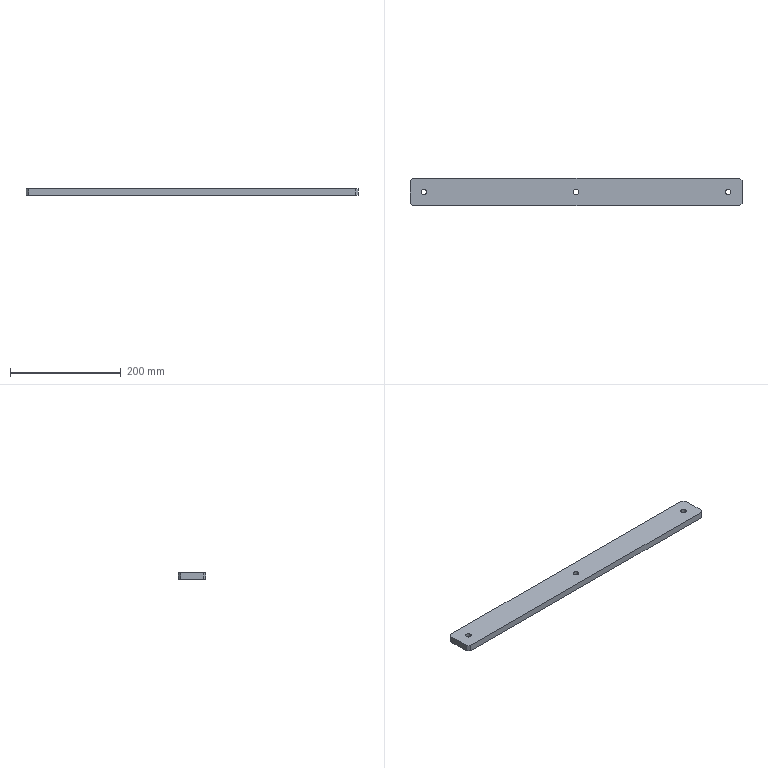Part | STEP file | [16] | 1 solid | 16 faces | box 600 x 50 x 12 mm | volume 356573 mm3 | plane 10 | cylinder 6 | commonest cylinder face diameters 10 x6
STEP:
#1=CARTESIAN_POINT('',(-530.,25.,0.));
#2=VERTEX_POINT('',#1);
#3=CARTESIAN_POINT('',(-520.,25.,0.));
#4=VERTEX_POINT('',#3);
#5=CARTESIAN_POINT('',(-525.,25.,0.));
#6=DIRECTION('',(0.,0.,1.));
#7=DIRECTION('',(1.,0.,0.));
#8=AXIS2_PLACEMENT_3D('',#5,#6,#7);
#9=CIRCLE('',#8,5.);
#10=EDGE_CURVE('',#2,#4,#9,.T.);
#11=ORIENTED_EDGE('',*,*,#10,.F.);
#12=CARTESIAN_POINT('',(-530.,25.,12.));
#13=VERTEX_POINT('',#12);
#14=CARTESIAN_POINT('',(-530.,25.,0.));
#15=DIRECTION('',(0.,0.,1.));
#16=VECTOR('',#15,1000.);
#17=LINE('',#14,#16);
#18=EDGE_CURVE('',#2,#13,#17,.T.);
#19=ORIENTED_EDGE('',*,*,#18,.T.);
#20=CARTESIAN_POINT('',(-520.,25.,12.));
#21=VERTEX_POINT('',#20);
#22=CARTESIAN_POINT('',(-525.,25.,12.));
#23=DIRECTION('',(0.,0.,-1.));
#24=DIRECTION('',(-1.,0.,0.));
#25=AXIS2_PLACEMENT_3D('',#22,#23,#24);
#26=CIRCLE('',#25,5.);
#27=EDGE_CURVE('',#21,#13,#26,.T.);
#28=ORIENTED_EDGE('',*,*,#27,.F.);
#29=CARTESIAN_POINT('',(-520.,25.,0.));
#30=DIRECTION('',(0.,0.,1.));
#31=VECTOR('',#30,1000.);
#32=LINE('',#29,#31);
#33=EDGE_CURVE('',#4,#21,#32,.T.);
#34=ORIENTED_EDGE('',*,*,#33,.F.);
#35=EDGE_LOOP('',(#11,#19,#28,#34));
#36=FACE_OUTER_BOUND('',#35,.T.);
#37=CARTESIAN_POINT('',(-525.,25.,0.));
#38=DIRECTION('',(0.,0.,1.));
#39=DIRECTION('',(1.,0.,0.));
#40=AXIS2_PLACEMENT_3D('',#37,#38,#39);
#41=CYLINDRICAL_SURFACE('',#40,5.);
#42=ADVANCED_FACE('',(#36),#41,.F.);
#43=CARTESIAN_POINT('',(-255.,25.,0.));
#44=VERTEX_POINT('',#43);
#45=CARTESIAN_POINT('',(-245.,25.,0.));
#46=VERTEX_POINT('',#45);
#47=CARTESIAN_POINT('',(-250.,25.,0.));
#48=DIRECTION('',(0.,0.,1.));
#49=DIRECTION('',(1.,0.,0.));
#50=AXIS2_PLACEMENT_3D('',#47,#48,#49);
#51=CIRCLE('',#50,5.);
#52=EDGE_CURVE('',#44,#46,#51,.T.);
#53=ORIENTED_EDGE('',*,*,#52,.F.);
#54=CARTESIAN_POINT('',(-255.,25.,12.));
#55=VERTEX_POINT('',#54);
#56=CARTESIAN_POINT('',(-255.,25.,0.));
#57=DIRECTION('',(0.,0.,1.));
#58=VECTOR('',#57,1000.);
#59=LINE('',#56,#58);
#60=EDGE_CURVE('',#44,#55,#59,.T.);
#61=ORIENTED_EDGE('',*,*,#60,.T.);
#62=CARTESIAN_POINT('',(-245.,25.,12.));
#63=VERTEX_POINT('',#62);
#64=CARTESIAN_POINT('',(-250.,25.,12.));
#65=DIRECTION('',(0.,0.,-1.));
#66=DIRECTION('',(-1.,0.,0.));
#67=AXIS2_PLACEMENT_3D('',#64,#65,#66);
#68=CIRCLE('',#67,5.);
#69=EDGE_CURVE('',#63,#55,#68,.T.);
#70=ORIENTED_EDGE('',*,*,#69,.F.);
#71=CARTESIAN_POINT('',(-245.,25.,0.));
#72=DIRECTION('',(0.,0.,1.));
#73=VECTOR('',#72,1000.);
#74=LINE('',#71,#73);
#75=EDGE_CURVE('',#46,#63,#74,.T.);
#76=ORIENTED_EDGE('',*,*,#75,.F.);
#77=EDGE_LOOP('',(#53,#61,#70,#76));
#78=FACE_OUTER_BOUND('',#77,.T.);
#79=CARTESIAN_POINT('',(-250.,25.,0.));
#80=DIRECTION('',(0.,0.,1.));
#81=DIRECTION('',(1.,0.,0.));
#82=AXIS2_PLACEMENT_3D('',#79,#80,#81);
#83=CYLINDRICAL_SURFACE('',#82,5.);
#84=ADVANCED_FACE('',(#78),#83,.F.);
#85=CARTESIAN_POINT('',(20.,25.,0.));
#86=VERTEX_POINT('',#85);
#87=CARTESIAN_POINT('',(30.,25.,0.));
#88=VERTEX_POINT('',#87);
#89=CARTESIAN_POINT('',(25.,25.,0.));
#90=DIRECTION('',(0.,0.,1.));
#91=DIRECTION('',(1.,0.,0.));
#92=AXIS2_PLACEMENT_3D('',#89,#90,#91);
#93=CIRCLE('',#92,5.);
#94=EDGE_CURVE('',#86,#88,#93,.T.);
#95=ORIENTED_EDGE('',*,*,#94,.F.);
#96=CARTESIAN_POINT('',(20.,25.,12.));
#97=VERTEX_POINT('',#96);
#98=CARTESIAN_POINT('',(20.,25.,0.));
#99=DIRECTION('',(0.,0.,1.));
#100=VECTOR('',#99,1000.);
#101=LINE('',#98,#100);
#102=EDGE_CURVE('',#86,#97,#101,.T.);
#103=ORIENTED_EDGE('',*,*,#102,.T.);
#104=CARTESIAN_POINT('',(30.,25.,12.));
#105=VERTEX_POINT('',#104);
#106=CARTESIAN_POINT('',(25.,25.,12.));
#107=DIRECTION('',(0.,0.,-1.));
#108=DIRECTION('',(-1.,0.,0.));
#109=AXIS2_PLACEMENT_3D('',#106,#107,#108);
#110=CIRCLE('',#109,5.);
#111=EDGE_CURVE('',#105,#97,#110,.T.);
#112=ORIENTED_EDGE('',*,*,#111,.F.);
#113=CARTESIAN_POINT('',(30.,25.,0.));
#114=DIRECTION('',(0.,0.,1.));
#115=VECTOR('',#114,1000.);
#116=LINE('',#113,#115);
#117=EDGE_CURVE('',#88,#105,#116,.T.);
#118=ORIENTED_EDGE('',*,*,#117,.F.);
#119=EDGE_LOOP('',(#95,#103,#112,#118));
#120=FACE_OUTER_BOUND('',#119,.T.);
#121=CARTESIAN_POINT('',(25.,25.,0.));
#122=DIRECTION('',(0.,0.,1.));
#123=DIRECTION('',(1.,0.,0.));
#124=AXIS2_PLACEMENT_3D('',#121,#122,#123);
#125=CYLINDRICAL_SURFACE('',#124,5.);
#126=ADVANCED_FACE('',(#120),#125,.F.);
#127=CARTESIAN_POINT('',(-525.,25.,0.));
#128=DIRECTION('',(0.,0.,1.));
#129=DIRECTION('',(1.,0.,0.));
#130=AXIS2_PLACEMENT_3D('',#127,#128,#129);
#131=CIRCLE('',#130,5.);
#132=EDGE_CURVE('',#4,#2,#131,.T.);
#133=ORIENTED_EDGE('',*,*,#132,.T.);
#134=ORIENTED_EDGE('',*,*,#10,.T.);
#135=EDGE_LOOP('',(#133,#134));
#136=FACE_BOUND('',#135,.T.);
#137=CARTESIAN_POINT('',(-250.,25.,0.));
#138=DIRECTION('',(0.,0.,1.));
#139=DIRECTION('',(1.,0.,0.));
#140=AXIS2_PLACEMENT_3D('',#137,#138,#139);
#141=CIRCLE('',#140,5.);
#142=EDGE_CURVE('',#46,#44,#141,.T.);
#143=ORIENTED_EDGE('',*,*,#142,.T.);
#144=ORIENTED_EDGE('',*,*,#52,.T.);
#145=EDGE_LOOP('',(#143,#144));
#146=FACE_BOUND('',#145,.T.);
#147=CARTESIAN_POINT('',(25.,25.,0.));
#148=DIRECTION('',(0.,0.,1.));
#149=DIRECTION('',(1.,0.,0.));
#150=AXIS2_PLACEMENT_3D('',#147,#148,#149);
#151=CIRCLE('',#150,5.);
#152=EDGE_CURVE('',#88,#86,#151,.T.);
#153=ORIENTED_EDGE('',*,*,#152,.T.);
#154=ORIENTED_EDGE('',*,*,#94,.T.);
#155=EDGE_LOOP('',(#153,#154));
#156=FACE_BOUND('',#155,.T.);
#157=CARTESIAN_POINT('',(-550.,45.,0.));
#158=VERTEX_POINT('',#157);
#159=CARTESIAN_POINT('',(-550.,5.,0.));
#160=VERTEX_POINT('',#159);
#161=CARTESIAN_POINT('',(-550.,25.,0.));
#162=DIRECTION('',(0.,-1.,0.));
#163=VECTOR('',#162,1000.);
#164=LINE('',#161,#163);
#165=EDGE_CURVE('',#158,#160,#164,.T.);
#166=ORIENTED_EDGE('',*,*,#165,.F.);
#167=CARTESIAN_POINT('',(-545.,50.,0.));
#168=VERTEX_POINT('',#167);
#169=CARTESIAN_POINT('',(-410.,185.,0.));
#170=DIRECTION('',(0.7071,0.7071,0.));
#171=VECTOR('',#170,1000.);
#172=LINE('',#169,#171);
#173=EDGE_CURVE('',#158,#168,#172,.T.);
#174=ORIENTED_EDGE('',*,*,#173,.T.);
#175=CARTESIAN_POINT('',(45.,50.,0.));
#176=VERTEX_POINT('',#175);
#177=CARTESIAN_POINT('',(-250.,50.,0.));
#178=DIRECTION('',(-1.,0.,0.));
#179=VECTOR('',#178,1000.);
#180=LINE('',#177,#179);
#181=EDGE_CURVE('',#176,#168,#180,.T.);
#182=ORIENTED_EDGE('',*,*,#181,.F.);
#183=CARTESIAN_POINT('',(50.,45.,0.));
#184=VERTEX_POINT('',#183);
#185=CARTESIAN_POINT('',(-90.,185.,0.));
#186=DIRECTION('',(0.7071,-0.7071,0.));
#187=VECTOR('',#186,1000.);
#188=LINE('',#185,#187);
#189=EDGE_CURVE('',#176,#184,#188,.T.);
#190=ORIENTED_EDGE('',*,*,#189,.T.);
#191=CARTESIAN_POINT('',(50.,5.,0.));
#192=VERTEX_POINT('',#191);
#193=CARTESIAN_POINT('',(50.,25.,0.));
#194=DIRECTION('',(0.,1.,0.));
#195=VECTOR('',#194,1000.);
#196=LINE('',#193,#195);
#197=EDGE_CURVE('',#192,#184,#196,.T.);
#198=ORIENTED_EDGE('',*,*,#197,.F.);
#199=CARTESIAN_POINT('',(45.,0.,0.));
#200=VERTEX_POINT('',#199);
#201=CARTESIAN_POINT('',(-90.,-135.,0.));
#202=DIRECTION('',(-0.7071,-0.7071,0.));
#203=VECTOR('',#202,1000.);
#204=LINE('',#201,#203);
#205=EDGE_CURVE('',#192,#200,#204,.T.);
#206=ORIENTED_EDGE('',*,*,#205,.T.);
#207=CARTESIAN_POINT('',(-545.,0.,0.));
#208=VERTEX_POINT('',#207);
#209=CARTESIAN_POINT('',(-250.,0.,0.));
#210=DIRECTION('',(1.,0.,0.));
#211=VECTOR('',#210,1000.);
#212=LINE('',#209,#211);
#213=EDGE_CURVE('',#208,#200,#212,.T.);
#214=ORIENTED_EDGE('',*,*,#213,.F.);
#215=CARTESIAN_POINT('',(-410.,-135.,0.));
#216=DIRECTION('',(-0.7071,0.7071,0.));
#217=VECTOR('',#216,1000.);
#218=LINE('',#215,#217);
#219=EDGE_CURVE('',#208,#160,#218,.T.);
#220=ORIENTED_EDGE('',*,*,#219,.T.);
#221=EDGE_LOOP('',(#166,#174,#182,#190,#198,#206,#214,#220));
#222=FACE_OUTER_BOUND('',#221,.T.);
#223=CARTESIAN_POINT('',(-250.,25.,0.));
#224=DIRECTION('',(0.,0.,-1.));
#225=DIRECTION('',(-1.,0.,0.));
#226=AXIS2_PLACEMENT_3D('',#223,#224,#225);
#227=PLANE('',#226);
#228=ADVANCED_FACE('',(#136,#146,#156,#222),#227,.T.);
#229=CARTESIAN_POINT('',(45.,0.,12.));
#230=VERTEX_POINT('',#229);
#231=CARTESIAN_POINT('',(-545.,0.,12.));
#232=VERTEX_POINT('',#231);
#233=CARTESIAN_POINT('',(-250.,0.,12.));
#234=DIRECTION('',(-1.,0.,0.));
#235=VECTOR('',#234,1000.);
#236=LINE('',#233,#235);
#237=EDGE_CURVE('',#230,#232,#236,.T.);
#238=ORIENTED_EDGE('',*,*,#237,.T.);
#239=CARTESIAN_POINT('',(-545.,0.,12.));
#240=DIRECTION('',(0.,0.,-1.));
#241=VECTOR('',#240,1000.);
#242=LINE('',#239,#241);
#243=EDGE_CURVE('',#232,#208,#242,.T.);
#244=ORIENTED_EDGE('',*,*,#243,.T.);
#245=ORIENTED_EDGE('',*,*,#213,.T.);
#246=CARTESIAN_POINT('',(45.,0.,12.));
#247=DIRECTION('',(0.,0.,1.));
#248=VECTOR('',#247,1000.);
#249=LINE('',#246,#248);
#250=EDGE_CURVE('',#200,#230,#249,.T.);
#251=ORIENTED_EDGE('',*,*,#250,.T.);
#252=EDGE_LOOP('',(#238,#244,#245,#251));
#253=FACE_OUTER_BOUND('',#252,.T.);
#254=CARTESIAN_POINT('',(-250.,0.,12.));
#255=DIRECTION('',(0.,-1.,0.));
#256=DIRECTION('',(0.,0.,1.));
#257=AXIS2_PLACEMENT_3D('',#254,#255,#256);
#258=PLANE('',#257);
#259=ADVANCED_FACE('',(#253),#258,.T.);
#260=CARTESIAN_POINT('',(50.,45.,12.));
#261=VERTEX_POINT('',#260);
#262=CARTESIAN_POINT('',(50.,5.,12.));
#263=VERTEX_POINT('',#262);
#264=CARTESIAN_POINT('',(50.,25.,12.));
#265=DIRECTION('',(0.,-1.,0.));
#266=VECTOR('',#265,1000.);
#267=LINE('',#264,#266);
#268=EDGE_CURVE('',#261,#263,#267,.T.);
#269=ORIENTED_EDGE('',*,*,#268,.T.);
#270=CARTESIAN_POINT('',(50.,5.,12.));
#271=DIRECTION('',(0.,0.,-1.));
#272=VECTOR('',#271,1000.);
#273=LINE('',#270,#272);
#274=EDGE_CURVE('',#263,#192,#273,.T.);
#275=ORIENTED_EDGE('',*,*,#274,.T.);
#276=ORIENTED_EDGE('',*,*,#197,.T.);
#277=CARTESIAN_POINT('',(50.,45.,12.));
#278=DIRECTION('',(0.,0.,1.));
#279=VECTOR('',#278,1000.);
#280=LINE('',#277,#279);
#281=EDGE_CURVE('',#184,#261,#280,.T.);
#282=ORIENTED_EDGE('',*,*,#281,.T.);
#283=EDGE_LOOP('',(#269,#275,#276,#282));
#284=FACE_OUTER_BOUND('',#283,.T.);
#285=CARTESIAN_POINT('',(50.,25.,12.));
#286=DIRECTION('',(1.,0.,0.));
#287=DIRECTION('',(0.,0.,-1.));
#288=AXIS2_PLACEMENT_3D('',#285,#286,#287);
#289=PLANE('',#288);
#290=ADVANCED_FACE('',(#284),#289,.T.);
#291=ORIENTED_EDGE('',*,*,#181,.T.);
#292=CARTESIAN_POINT('',(-545.,50.,12.));
#293=VERTEX_POINT('',#292);
#294=CARTESIAN_POINT('',(-545.,50.,12.));
#295=DIRECTION('',(0.,0.,1.));
#296=VECTOR('',#295,1000.);
#297=LINE('',#294,#296);
#298=EDGE_CURVE('',#168,#293,#297,.T.);
#299=ORIENTED_EDGE('',*,*,#298,.T.);
#300=CARTESIAN_POINT('',(45.,50.,12.));
#301=VERTEX_POINT('',#300);
#302=CARTESIAN_POINT('',(-250.,50.,12.));
#303=DIRECTION('',(1.,0.,0.));
#304=VECTOR('',#303,1000.);
#305=LINE('',#302,#304);
#306=EDGE_CURVE('',#293,#301,#305,.T.);
#307=ORIENTED_EDGE('',*,*,#306,.T.);
#308=CARTESIAN_POINT('',(45.,50.,12.));
#309=DIRECTION('',(0.,0.,-1.));
#310=VECTOR('',#309,1000.);
#311=LINE('',#308,#310);
#312=EDGE_CURVE('',#301,#176,#311,.T.);
#313=ORIENTED_EDGE('',*,*,#312,.T.);
#314=EDGE_LOOP('',(#291,#299,#307,#313));
#315=FACE_OUTER_BOUND('',#314,.T.);
#316=CARTESIAN_POINT('',(-250.,50.,12.));
#317=DIRECTION('',(0.,1.,0.));
#318=DIRECTION('',(0.,0.,-1.));
#319=AXIS2_PLACEMENT_3D('',#316,#317,#318);
#320=PLANE('',#319);
#321=ADVANCED_FACE('',(#315),#320,.T.);
#322=ORIENTED_EDGE('',*,*,#27,.T.);
#323=CARTESIAN_POINT('',(-525.,25.,12.));
#324=DIRECTION('',(0.,0.,-1.));
#325=DIRECTION('',(-1.,0.,0.));
#326=AXIS2_PLACEMENT_3D('',#323,#324,#325);
#327=CIRCLE('',#326,5.);
#328=EDGE_CURVE('',#13,#21,#327,.T.);
#329=ORIENTED_EDGE('',*,*,#328,.T.);
#330=EDGE_LOOP('',(#322,#329));
#331=FACE_BOUND('',#330,.T.);
#332=ORIENTED_EDGE('',*,*,#69,.T.);
#333=CARTESIAN_POINT('',(-250.,25.,12.));
#334=DIRECTION('',(0.,0.,-1.));
#335=DIRECTION('',(-1.,0.,0.));
#336=AXIS2_PLACEMENT_3D('',#333,#334,#335);
#337=CIRCLE('',#336,5.);
#338=EDGE_CURVE('',#55,#63,#337,.T.);
#339=ORIENTED_EDGE('',*,*,#338,.T.);
#340=EDGE_LOOP('',(#332,#339));
#341=FACE_BOUND('',#340,.T.);
#342=ORIENTED_EDGE('',*,*,#111,.T.);
#343=CARTESIAN_POINT('',(25.,25.,12.));
#344=DIRECTION('',(0.,0.,-1.));
#345=DIRECTION('',(-1.,0.,0.));
#346=AXIS2_PLACEMENT_3D('',#343,#344,#345);
#347=CIRCLE('',#346,5.);
#348=EDGE_CURVE('',#97,#105,#347,.T.);
#349=ORIENTED_EDGE('',*,*,#348,.T.);
#350=EDGE_LOOP('',(#342,#349));
#351=FACE_BOUND('',#350,.T.);
#352=ORIENTED_EDGE('',*,*,#306,.F.);
#353=CARTESIAN_POINT('',(-550.,45.,12.));
#354=VERTEX_POINT('',#353);
#355=CARTESIAN_POINT('',(-410.,185.,12.));
#356=DIRECTION('',(-0.7071,-0.7071,0.));
#357=VECTOR('',#356,1000.);
#358=LINE('',#355,#357);
#359=EDGE_CURVE('',#293,#354,#358,.T.);
#360=ORIENTED_EDGE('',*,*,#359,.T.);
#361=CARTESIAN_POINT('',(-550.,5.,12.));
#362=VERTEX_POINT('',#361);
#363=CARTESIAN_POINT('',(-550.,25.,12.));
#364=DIRECTION('',(0.,1.,0.));
#365=VECTOR('',#364,1000.);
#366=LINE('',#363,#365);
#367=EDGE_CURVE('',#362,#354,#366,.T.);
#368=ORIENTED_EDGE('',*,*,#367,.F.);
#369=CARTESIAN_POINT('',(-410.,-135.,12.));
#370=DIRECTION('',(0.7071,-0.7071,0.));
#371=VECTOR('',#370,1000.);
#372=LINE('',#369,#371);
#373=EDGE_CURVE('',#362,#232,#372,.T.);
#374=ORIENTED_EDGE('',*,*,#373,.T.);
#375=ORIENTED_EDGE('',*,*,#237,.F.);
#376=CARTESIAN_POINT('',(-90.,-135.,12.));
#377=DIRECTION('',(0.7071,0.7071,0.));
#378=VECTOR('',#377,1000.);
#379=LINE('',#376,#378);
#380=EDGE_CURVE('',#230,#263,#379,.T.);
#381=ORIENTED_EDGE('',*,*,#380,.T.);
#382=ORIENTED_EDGE('',*,*,#268,.F.);
#383=CARTESIAN_POINT('',(-90.,185.,12.));
#384=DIRECTION('',(-0.7071,0.7071,0.));
#385=VECTOR('',#384,1000.);
#386=LINE('',#383,#385);
#387=EDGE_CURVE('',#261,#301,#386,.T.);
#388=ORIENTED_EDGE('',*,*,#387,.T.);
#389=EDGE_LOOP('',(#352,#360,#368,#374,#375,#381,#382,#388));
#390=FACE_OUTER_BOUND('',#389,.T.);
#391=CARTESIAN_POINT('',(-250.,25.,12.));
#392=DIRECTION('',(0.,0.,1.));
#393=DIRECTION('',(1.,0.,0.));
#394=AXIS2_PLACEMENT_3D('',#391,#392,#393);
#395=PLANE('',#394);
#396=ADVANCED_FACE('',(#331,#341,#351,#390),#395,.T.);
#397=ORIENTED_EDGE('',*,*,#367,.T.);
#398=CARTESIAN_POINT('',(-550.,45.,12.));
#399=DIRECTION('',(0.,0.,-1.));
#400=VECTOR('',#399,1000.);
#401=LINE('',#398,#400);
#402=EDGE_CURVE('',#354,#158,#401,.T.);
#403=ORIENTED_EDGE('',*,*,#402,.T.);
#404=ORIENTED_EDGE('',*,*,#165,.T.);
#405=CARTESIAN_POINT('',(-550.,5.,12.));
#406=DIRECTION('',(0.,0.,1.));
#407=VECTOR('',#406,1000.);
#408=LINE('',#405,#407);
#409=EDGE_CURVE('',#160,#362,#408,.T.);
#410=ORIENTED_EDGE('',*,*,#409,.T.);
#411=EDGE_LOOP('',(#397,#403,#404,#410));
#412=FACE_OUTER_BOUND('',#411,.T.);
#413=CARTESIAN_POINT('',(-550.,25.,12.));
#414=DIRECTION('',(-1.,0.,0.));
#415=DIRECTION('',(0.,0.,1.));
#416=AXIS2_PLACEMENT_3D('',#413,#414,#415);
#417=PLANE('',#416);
#418=ADVANCED_FACE('',(#412),#417,.T.);
#419=ORIENTED_EDGE('',*,*,#102,.F.);
#420=ORIENTED_EDGE('',*,*,#152,.F.);
#421=ORIENTED_EDGE('',*,*,#117,.T.);
#422=ORIENTED_EDGE('',*,*,#348,.F.);
#423=EDGE_LOOP('',(#419,#420,#421,#422));
#424=FACE_OUTER_BOUND('',#423,.T.);
#425=CARTESIAN_POINT('',(25.,25.,0.));
#426=DIRECTION('',(0.,0.,1.));
#427=DIRECTION('',(1.,0.,0.));
#428=AXIS2_PLACEMENT_3D('',#425,#426,#427);
#429=CYLINDRICAL_SURFACE('',#428,5.);
#430=ADVANCED_FACE('',(#424),#429,.F.);
#431=ORIENTED_EDGE('',*,*,#359,.F.);
#432=ORIENTED_EDGE('',*,*,#298,.F.);
#433=ORIENTED_EDGE('',*,*,#173,.F.);
#434=ORIENTED_EDGE('',*,*,#402,.F.);
#435=EDGE_LOOP('',(#431,#432,#433,#434));
#436=FACE_OUTER_BOUND('',#435,.T.);
#437=CARTESIAN_POINT('',(-550.,45.,12.));
#438=DIRECTION('',(0.7071,-0.7071,0.));
#439=DIRECTION('',(0.,0.,-1.));
#440=AXIS2_PLACEMENT_3D('',#437,#438,#439);
#441=PLANE('',#440);
#442=ADVANCED_FACE('',(#436),#441,.F.);
#443=ORIENTED_EDGE('',*,*,#373,.F.);
#444=ORIENTED_EDGE('',*,*,#409,.F.);
#445=ORIENTED_EDGE('',*,*,#219,.F.);
#446=ORIENTED_EDGE('',*,*,#243,.F.);
#447=EDGE_LOOP('',(#443,#444,#445,#446));
#448=FACE_OUTER_BOUND('',#447,.T.);
#449=CARTESIAN_POINT('',(-545.,0.,12.));
#450=DIRECTION('',(0.7071,0.7071,0.));
#451=DIRECTION('',(0.,0.,-1.));
#452=AXIS2_PLACEMENT_3D('',#449,#450,#451);
#453=PLANE('',#452);
#454=ADVANCED_FACE('',(#448),#453,.F.);
#455=ORIENTED_EDGE('',*,*,#380,.F.);
#456=ORIENTED_EDGE('',*,*,#250,.F.);
#457=ORIENTED_EDGE('',*,*,#205,.F.);
#458=ORIENTED_EDGE('',*,*,#274,.F.);
#459=EDGE_LOOP('',(#455,#456,#457,#458));
#460=FACE_OUTER_BOUND('',#459,.T.);
#461=CARTESIAN_POINT('',(50.,5.,12.));
#462=DIRECTION('',(-0.7071,0.7071,0.));
#463=DIRECTION('',(0.,0.,-1.));
#464=AXIS2_PLACEMENT_3D('',#461,#462,#463);
#465=PLANE('',#464);
#466=ADVANCED_FACE('',(#460),#465,.F.);
#467=ORIENTED_EDGE('',*,*,#387,.F.);
#468=ORIENTED_EDGE('',*,*,#281,.F.);
#469=ORIENTED_EDGE('',*,*,#189,.F.);
#470=ORIENTED_EDGE('',*,*,#312,.F.);
#471=EDGE_LOOP('',(#467,#468,#469,#470));
#472=FACE_OUTER_BOUND('',#471,.T.);
#473=CARTESIAN_POINT('',(45.,50.,12.));
#474=DIRECTION('',(-0.7071,-0.7071,0.));
#475=DIRECTION('',(0.,0.,-1.));
#476=AXIS2_PLACEMENT_3D('',#473,#474,#475);
#477=PLANE('',#476);
#478=ADVANCED_FACE('',(#472),#477,.F.);
#479=ORIENTED_EDGE('',*,*,#60,.F.);
#480=ORIENTED_EDGE('',*,*,#142,.F.);
#481=ORIENTED_EDGE('',*,*,#75,.T.);
#482=ORIENTED_EDGE('',*,*,#338,.F.);
#483=EDGE_LOOP('',(#479,#480,#481,#482));
#484=FACE_OUTER_BOUND('',#483,.T.);
#485=CARTESIAN_POINT('',(-250.,25.,0.));
#486=DIRECTION('',(0.,0.,1.));
#487=DIRECTION('',(1.,0.,0.));
#488=AXIS2_PLACEMENT_3D('',#485,#486,#487);
#489=CYLINDRICAL_SURFACE('',#488,5.);
#490=ADVANCED_FACE('',(#484),#489,.F.);
#491=ORIENTED_EDGE('',*,*,#18,.F.);
#492=ORIENTED_EDGE('',*,*,#132,.F.);
#493=ORIENTED_EDGE('',*,*,#33,.T.);
#494=ORIENTED_EDGE('',*,*,#328,.F.);
#495=EDGE_LOOP('',(#491,#492,#493,#494));
#496=FACE_OUTER_BOUND('',#495,.T.);
#497=CARTESIAN_POINT('',(-525.,25.,0.));
#498=DIRECTION('',(0.,0.,1.));
#499=DIRECTION('',(1.,0.,0.));
#500=AXIS2_PLACEMENT_3D('',#497,#498,#499);
#501=CYLINDRICAL_SURFACE('',#500,5.);
#502=ADVANCED_FACE('',(#496),#501,.F.);
#503=CLOSED_SHELL('',(#42,#84,#126,#228,#259,#290,#321,#396,#418,#430,#442,#454,#466,#478,#490,#502));
#504=MANIFOLD_SOLID_BREP('',#503);
#505=CARTESIAN_POINT('',(0.,0.,0.));
#506=DIRECTION('',(0.,0.,1.));
#507=DIRECTION('',(1.,0.,0.));
#508=AXIS2_PLACEMENT_3D('',#505,#506,#507);
#509=(LENGTH_UNIT()NAMED_UNIT(*)SI_UNIT(.MILLI.,.METRE.));
#510=UNCERTAINTY_MEASURE_WITH_UNIT(LENGTH_MEASURE(0.00001),#509,'','');
#511=(NAMED_UNIT(*)PLANE_ANGLE_UNIT()SI_UNIT($,.RADIAN.));
#512=(NAMED_UNIT(*)SI_UNIT($,.STERADIAN.)SOLID_ANGLE_UNIT());
#513=(GEOMETRIC_REPRESENTATION_CONTEXT(3)GLOBAL_UNCERTAINTY_ASSIGNED_CONTEXT((#510))GLOBAL_UNIT_ASSIGNED_CONTEXT((#509,#511,#512))REPRESENTATION_CONTEXT('',''));
#514=ADVANCED_BREP_SHAPE_REPRESENTATION('',(#504,#508),#513);